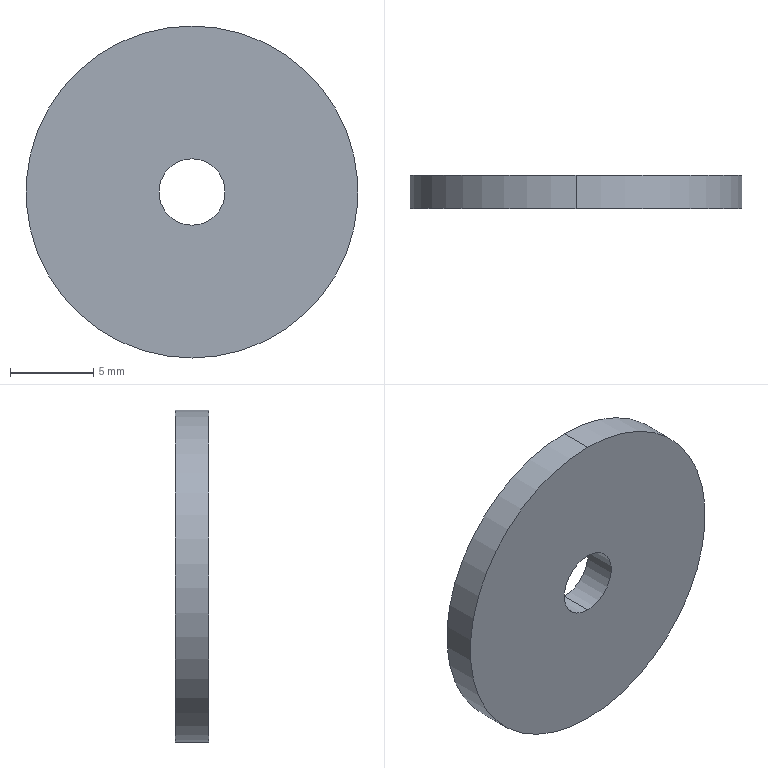Part | SolidWorks | features Extrusion 1 | 1 solid | 6 faces | box 20 x 2 x 20 mm | volume 603.186 mm3 | cylinder 4 | plane 2 | commonest cylinder face diameters 4 x2 20 x2
STEP:
#1=CARTESIAN_POINT('',(0.,2.,-2.));
#2=VERTEX_POINT('',#1);
#3=CARTESIAN_POINT('',(0.,2.,2.));
#4=VERTEX_POINT('',#3);
#5=CARTESIAN_POINT('',(0.,2.,0.));
#6=DIRECTION('',(0.,1.,0.));
#7=DIRECTION('',(0.,0.,1.));
#8=AXIS2_PLACEMENT_3D('',#5,#6,#7);
#9=CIRCLE('',#8,2.);
#10=EDGE_CURVE('',#2,#4,#9,.T.);
#11=ORIENTED_EDGE('',*,*,#10,.T.);
#12=CARTESIAN_POINT('',(0.,0.,2.));
#13=VERTEX_POINT('',#12);
#14=CARTESIAN_POINT('',(0.,2.,2.));
#15=DIRECTION('',(0.,-1.,0.));
#16=VECTOR('',#15,1000.);
#17=LINE('',#14,#16);
#18=EDGE_CURVE('',#4,#13,#17,.T.);
#19=ORIENTED_EDGE('',*,*,#18,.T.);
#20=CARTESIAN_POINT('',(0.,0.,-2.));
#21=VERTEX_POINT('',#20);
#22=CARTESIAN_POINT('',(0.,0.,0.));
#23=DIRECTION('',(0.,1.,0.));
#24=DIRECTION('',(0.,0.,1.));
#25=AXIS2_PLACEMENT_3D('',#22,#23,#24);
#26=CIRCLE('',#25,2.);
#27=EDGE_CURVE('',#21,#13,#26,.T.);
#28=ORIENTED_EDGE('',*,*,#27,.F.);
#29=CARTESIAN_POINT('',(0.,2.,-2.));
#30=DIRECTION('',(0.,-1.,0.));
#31=VECTOR('',#30,1000.);
#32=LINE('',#29,#31);
#33=EDGE_CURVE('',#2,#21,#32,.T.);
#34=ORIENTED_EDGE('',*,*,#33,.F.);
#35=EDGE_LOOP('',(#11,#19,#28,#34));
#36=FACE_OUTER_BOUND('',#35,.T.);
#37=CARTESIAN_POINT('',(0.,2.,0.));
#38=DIRECTION('',(0.,-1.,0.));
#39=DIRECTION('',(0.,0.,-1.));
#40=AXIS2_PLACEMENT_3D('',#37,#38,#39);
#41=CYLINDRICAL_SURFACE('',#40,2.);
#42=ADVANCED_FACE('',(#36),#41,.F.);
#43=CARTESIAN_POINT('',(0.,2.,10.));
#44=VERTEX_POINT('',#43);
#45=CARTESIAN_POINT('',(0.,2.,-10.));
#46=VERTEX_POINT('',#45);
#47=CARTESIAN_POINT('',(0.,2.,0.));
#48=DIRECTION('',(0.,1.,0.));
#49=DIRECTION('',(0.,0.,1.));
#50=AXIS2_PLACEMENT_3D('',#47,#48,#49);
#51=CIRCLE('',#50,10.);
#52=EDGE_CURVE('',#44,#46,#51,.T.);
#53=ORIENTED_EDGE('',*,*,#52,.F.);
#54=CARTESIAN_POINT('',(0.,0.,10.));
#55=VERTEX_POINT('',#54);
#56=CARTESIAN_POINT('',(0.,2.,10.));
#57=DIRECTION('',(0.,-1.,0.));
#58=VECTOR('',#57,1000.);
#59=LINE('',#56,#58);
#60=EDGE_CURVE('',#44,#55,#59,.T.);
#61=ORIENTED_EDGE('',*,*,#60,.T.);
#62=CARTESIAN_POINT('',(0.,0.,-10.));
#63=VERTEX_POINT('',#62);
#64=CARTESIAN_POINT('',(0.,0.,0.));
#65=DIRECTION('',(0.,1.,0.));
#66=DIRECTION('',(0.,0.,1.));
#67=AXIS2_PLACEMENT_3D('',#64,#65,#66);
#68=CIRCLE('',#67,10.);
#69=EDGE_CURVE('',#55,#63,#68,.T.);
#70=ORIENTED_EDGE('',*,*,#69,.T.);
#71=CARTESIAN_POINT('',(0.,2.,-10.));
#72=DIRECTION('',(0.,-1.,0.));
#73=VECTOR('',#72,1000.);
#74=LINE('',#71,#73);
#75=EDGE_CURVE('',#46,#63,#74,.T.);
#76=ORIENTED_EDGE('',*,*,#75,.F.);
#77=EDGE_LOOP('',(#53,#61,#70,#76));
#78=FACE_OUTER_BOUND('',#77,.T.);
#79=CARTESIAN_POINT('',(0.,2.,0.));
#80=DIRECTION('',(0.,-1.,0.));
#81=DIRECTION('',(0.,0.,-1.));
#82=AXIS2_PLACEMENT_3D('',#79,#80,#81);
#83=CYLINDRICAL_SURFACE('',#82,10.);
#84=ADVANCED_FACE('',(#78),#83,.T.);
#85=CARTESIAN_POINT('',(0.,2.,0.));
#86=DIRECTION('',(0.,1.,0.));
#87=DIRECTION('',(0.,0.,1.));
#88=AXIS2_PLACEMENT_3D('',#85,#86,#87);
#89=CIRCLE('',#88,10.);
#90=EDGE_CURVE('',#46,#44,#89,.T.);
#91=ORIENTED_EDGE('',*,*,#90,.T.);
#92=ORIENTED_EDGE('',*,*,#52,.T.);
#93=EDGE_LOOP('',(#91,#92));
#94=FACE_OUTER_BOUND('',#93,.T.);
#95=ORIENTED_EDGE('',*,*,#10,.F.);
#96=CARTESIAN_POINT('',(0.,2.,0.));
#97=DIRECTION('',(0.,1.,0.));
#98=DIRECTION('',(0.,0.,1.));
#99=AXIS2_PLACEMENT_3D('',#96,#97,#98);
#100=CIRCLE('',#99,2.);
#101=EDGE_CURVE('',#4,#2,#100,.T.);
#102=ORIENTED_EDGE('',*,*,#101,.F.);
#103=EDGE_LOOP('',(#95,#102));
#104=FACE_BOUND('',#103,.T.);
#105=CARTESIAN_POINT('',(0.,2.,0.));
#106=DIRECTION('',(0.,1.,0.));
#107=DIRECTION('',(0.,0.,1.));
#108=AXIS2_PLACEMENT_3D('',#105,#106,#107);
#109=PLANE('',#108);
#110=ADVANCED_FACE('',(#94,#104),#109,.T.);
#111=CARTESIAN_POINT('',(0.,0.,0.));
#112=DIRECTION('',(0.,1.,0.));
#113=DIRECTION('',(0.,0.,1.));
#114=AXIS2_PLACEMENT_3D('',#111,#112,#113);
#115=CIRCLE('',#114,10.);
#116=EDGE_CURVE('',#63,#55,#115,.T.);
#117=ORIENTED_EDGE('',*,*,#116,.F.);
#118=ORIENTED_EDGE('',*,*,#69,.F.);
#119=EDGE_LOOP('',(#117,#118));
#120=FACE_OUTER_BOUND('',#119,.T.);
#121=ORIENTED_EDGE('',*,*,#27,.T.);
#122=CARTESIAN_POINT('',(0.,0.,0.));
#123=DIRECTION('',(0.,1.,0.));
#124=DIRECTION('',(0.,0.,1.));
#125=AXIS2_PLACEMENT_3D('',#122,#123,#124);
#126=CIRCLE('',#125,2.);
#127=EDGE_CURVE('',#13,#21,#126,.T.);
#128=ORIENTED_EDGE('',*,*,#127,.T.);
#129=EDGE_LOOP('',(#121,#128));
#130=FACE_BOUND('',#129,.T.);
#131=CARTESIAN_POINT('',(0.,0.,0.));
#132=DIRECTION('',(0.,1.,0.));
#133=DIRECTION('',(0.,0.,1.));
#134=AXIS2_PLACEMENT_3D('',#131,#132,#133);
#135=PLANE('',#134);
#136=ADVANCED_FACE('',(#120,#130),#135,.F.);
#137=ORIENTED_EDGE('',*,*,#60,.F.);
#138=ORIENTED_EDGE('',*,*,#90,.F.);
#139=ORIENTED_EDGE('',*,*,#75,.T.);
#140=ORIENTED_EDGE('',*,*,#116,.T.);
#141=EDGE_LOOP('',(#137,#138,#139,#140));
#142=FACE_OUTER_BOUND('',#141,.T.);
#143=CARTESIAN_POINT('',(0.,2.,0.));
#144=DIRECTION('',(0.,-1.,0.));
#145=DIRECTION('',(0.,0.,-1.));
#146=AXIS2_PLACEMENT_3D('',#143,#144,#145);
#147=CYLINDRICAL_SURFACE('',#146,10.);
#148=ADVANCED_FACE('',(#142),#147,.T.);
#149=ORIENTED_EDGE('',*,*,#18,.F.);
#150=ORIENTED_EDGE('',*,*,#101,.T.);
#151=ORIENTED_EDGE('',*,*,#33,.T.);
#152=ORIENTED_EDGE('',*,*,#127,.F.);
#153=EDGE_LOOP('',(#149,#150,#151,#152));
#154=FACE_OUTER_BOUND('',#153,.T.);
#155=CARTESIAN_POINT('',(0.,2.,0.));
#156=DIRECTION('',(0.,-1.,0.));
#157=DIRECTION('',(0.,0.,-1.));
#158=AXIS2_PLACEMENT_3D('',#155,#156,#157);
#159=CYLINDRICAL_SURFACE('',#158,2.);
#160=ADVANCED_FACE('',(#154),#159,.F.);
#161=CLOSED_SHELL('',(#42,#84,#110,#136,#148,#160));
#162=MANIFOLD_SOLID_BREP('',#161);
#163=CARTESIAN_POINT('',(0.,0.,0.));
#164=DIRECTION('',(0.,0.,1.));
#165=DIRECTION('',(1.,0.,0.));
#166=AXIS2_PLACEMENT_3D('',#163,#164,#165);
#167=(LENGTH_UNIT()NAMED_UNIT(*)SI_UNIT(.MILLI.,.METRE.));
#168=UNCERTAINTY_MEASURE_WITH_UNIT(LENGTH_MEASURE(0.00001),#167,'','');
#169=(NAMED_UNIT(*)PLANE_ANGLE_UNIT()SI_UNIT($,.RADIAN.));
#170=(NAMED_UNIT(*)SI_UNIT($,.STERADIAN.)SOLID_ANGLE_UNIT());
#171=(GEOMETRIC_REPRESENTATION_CONTEXT(3)GLOBAL_UNCERTAINTY_ASSIGNED_CONTEXT((#168))GLOBAL_UNIT_ASSIGNED_CONTEXT((#167,#169,#170))REPRESENTATION_CONTEXT('',''));
#172=ADVANCED_BREP_SHAPE_REPRESENTATION('',(#162,#166),#171);